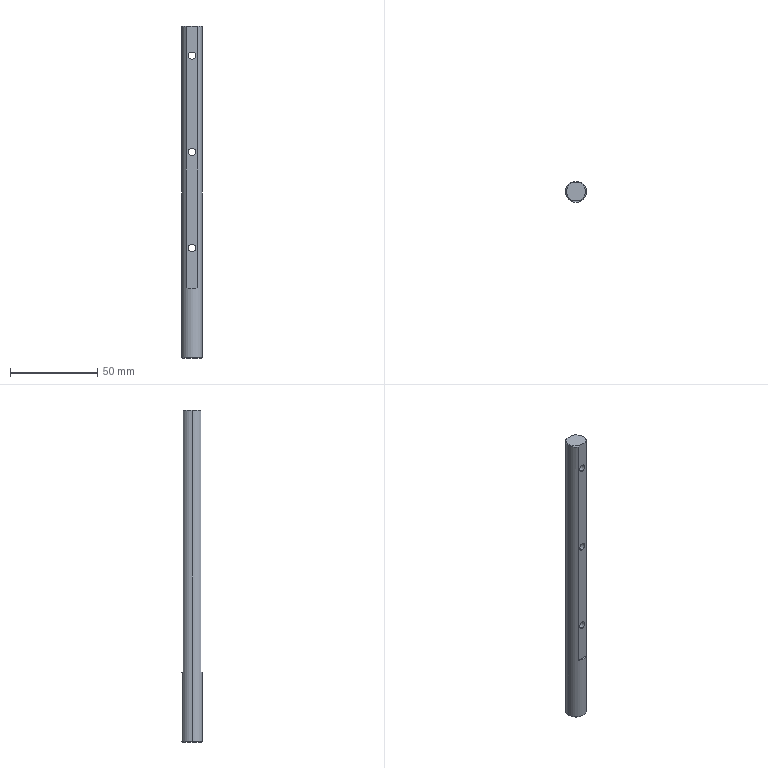Part | STEP file | 11-FG-S00411 | 1 solid | 19 faces | box 12 x 12 x 190 mm | volume 19715 mm3 | cylinder 8 | plane 6 | cone 5 | commonest cylinder face diameters 4.2 x6 12 x2
STEP:
#1=CARTESIAN_POINT('',(0.,-5.,75.9));
#2=VERTEX_POINT('',#1);
#3=CARTESIAN_POINT('',(0.,-5.,80.1));
#4=VERTEX_POINT('',#3);
#5=CARTESIAN_POINT('',(0.,-5.,78.));
#6=DIRECTION('',(0.,1.,0.));
#7=DIRECTION('',(0.,0.,1.));
#8=AXIS2_PLACEMENT_3D('',#5,#6,#7);
#9=CIRCLE('',#8,2.1);
#10=EDGE_CURVE('',#2,#4,#9,.T.);
#11=ORIENTED_EDGE('',*,*,#10,.F.);
#12=CARTESIAN_POINT('',(0.,5.,75.9));
#13=VERTEX_POINT('',#12);
#14=CARTESIAN_POINT('',(0.,-123.,75.9));
#15=DIRECTION('',(0.,1.,0.));
#16=VECTOR('',#15,1000.);
#17=LINE('',#14,#16);
#18=EDGE_CURVE('',#2,#13,#17,.T.);
#19=ORIENTED_EDGE('',*,*,#18,.T.);
#20=CARTESIAN_POINT('',(0.,5.,80.1));
#21=VERTEX_POINT('',#20);
#22=CARTESIAN_POINT('',(0.,5.,78.));
#23=DIRECTION('',(0.,1.,0.));
#24=DIRECTION('',(0.,0.,1.));
#25=AXIS2_PLACEMENT_3D('',#22,#23,#24);
#26=CIRCLE('',#25,2.1);
#27=EDGE_CURVE('',#13,#21,#26,.T.);
#28=ORIENTED_EDGE('',*,*,#27,.T.);
#29=CARTESIAN_POINT('',(0.,-123.,80.1));
#30=DIRECTION('',(0.,1.,0.));
#31=VECTOR('',#30,1000.);
#32=LINE('',#29,#31);
#33=EDGE_CURVE('',#4,#21,#32,.T.);
#34=ORIENTED_EDGE('',*,*,#33,.F.);
#35=EDGE_LOOP('',(#11,#19,#28,#34));
#36=FACE_OUTER_BOUND('',#35,.T.);
#37=CARTESIAN_POINT('',(0.,-123.,78.));
#38=DIRECTION('',(0.,1.,0.));
#39=DIRECTION('',(0.,0.,1.));
#40=AXIS2_PLACEMENT_3D('',#37,#38,#39);
#41=CYLINDRICAL_SURFACE('',#40,2.1);
#42=ADVANCED_FACE('',(#36),#41,.F.);
#43=CARTESIAN_POINT('',(0.,-5.,20.9));
#44=VERTEX_POINT('',#43);
#45=CARTESIAN_POINT('',(0.,-5.,25.1));
#46=VERTEX_POINT('',#45);
#47=CARTESIAN_POINT('',(0.,-5.,23.));
#48=DIRECTION('',(0.,1.,0.));
#49=DIRECTION('',(0.,0.,1.));
#50=AXIS2_PLACEMENT_3D('',#47,#48,#49);
#51=CIRCLE('',#50,2.1);
#52=EDGE_CURVE('',#44,#46,#51,.T.);
#53=ORIENTED_EDGE('',*,*,#52,.F.);
#54=CARTESIAN_POINT('',(0.,5.,20.9));
#55=VERTEX_POINT('',#54);
#56=CARTESIAN_POINT('',(0.,-123.,20.9));
#57=DIRECTION('',(0.,1.,0.));
#58=VECTOR('',#57,1000.);
#59=LINE('',#56,#58);
#60=EDGE_CURVE('',#44,#55,#59,.T.);
#61=ORIENTED_EDGE('',*,*,#60,.T.);
#62=CARTESIAN_POINT('',(0.,5.,25.1));
#63=VERTEX_POINT('',#62);
#64=CARTESIAN_POINT('',(0.,5.,23.));
#65=DIRECTION('',(0.,1.,0.));
#66=DIRECTION('',(0.,0.,1.));
#67=AXIS2_PLACEMENT_3D('',#64,#65,#66);
#68=CIRCLE('',#67,2.1);
#69=EDGE_CURVE('',#55,#63,#68,.T.);
#70=ORIENTED_EDGE('',*,*,#69,.T.);
#71=CARTESIAN_POINT('',(0.,-123.,25.1));
#72=DIRECTION('',(0.,1.,0.));
#73=VECTOR('',#72,1000.);
#74=LINE('',#71,#73);
#75=EDGE_CURVE('',#46,#63,#74,.T.);
#76=ORIENTED_EDGE('',*,*,#75,.F.);
#77=EDGE_LOOP('',(#53,#61,#70,#76));
#78=FACE_OUTER_BOUND('',#77,.T.);
#79=CARTESIAN_POINT('',(0.,-123.,23.));
#80=DIRECTION('',(0.,1.,0.));
#81=DIRECTION('',(0.,0.,1.));
#82=AXIS2_PLACEMENT_3D('',#79,#80,#81);
#83=CYLINDRICAL_SURFACE('',#82,2.1);
#84=ADVANCED_FACE('',(#78),#83,.F.);
#85=CARTESIAN_POINT('',(0.,-5.,-34.1));
#86=VERTEX_POINT('',#85);
#87=CARTESIAN_POINT('',(0.,-5.,-29.9));
#88=VERTEX_POINT('',#87);
#89=CARTESIAN_POINT('',(0.,-5.,-32.));
#90=DIRECTION('',(0.,1.,0.));
#91=DIRECTION('',(0.,0.,1.));
#92=AXIS2_PLACEMENT_3D('',#89,#90,#91);
#93=CIRCLE('',#92,2.1);
#94=EDGE_CURVE('',#86,#88,#93,.T.);
#95=ORIENTED_EDGE('',*,*,#94,.F.);
#96=CARTESIAN_POINT('',(0.,5.,-34.1));
#97=VERTEX_POINT('',#96);
#98=CARTESIAN_POINT('',(0.,-123.,-34.1));
#99=DIRECTION('',(0.,1.,0.));
#100=VECTOR('',#99,1000.);
#101=LINE('',#98,#100);
#102=EDGE_CURVE('',#86,#97,#101,.T.);
#103=ORIENTED_EDGE('',*,*,#102,.T.);
#104=CARTESIAN_POINT('',(0.,5.,-29.9));
#105=VERTEX_POINT('',#104);
#106=CARTESIAN_POINT('',(0.,5.,-32.));
#107=DIRECTION('',(0.,1.,0.));
#108=DIRECTION('',(0.,0.,1.));
#109=AXIS2_PLACEMENT_3D('',#106,#107,#108);
#110=CIRCLE('',#109,2.1);
#111=EDGE_CURVE('',#97,#105,#110,.T.);
#112=ORIENTED_EDGE('',*,*,#111,.T.);
#113=CARTESIAN_POINT('',(0.,-123.,-29.9));
#114=DIRECTION('',(0.,1.,0.));
#115=VECTOR('',#114,1000.);
#116=LINE('',#113,#115);
#117=EDGE_CURVE('',#88,#105,#116,.T.);
#118=ORIENTED_EDGE('',*,*,#117,.F.);
#119=EDGE_LOOP('',(#95,#103,#112,#118));
#120=FACE_OUTER_BOUND('',#119,.T.);
#121=CARTESIAN_POINT('',(0.,-123.,-32.));
#122=DIRECTION('',(0.,1.,0.));
#123=DIRECTION('',(0.,0.,1.));
#124=AXIS2_PLACEMENT_3D('',#121,#122,#123);
#125=CYLINDRICAL_SURFACE('',#124,2.1);
#126=ADVANCED_FACE('',(#120),#125,.F.);
#127=CARTESIAN_POINT('',(-5.5,0.,-95.));
#128=VERTEX_POINT('',#127);
#129=CARTESIAN_POINT('',(5.5,0.,-95.));
#130=VERTEX_POINT('',#129);
#131=CARTESIAN_POINT('',(0.,0.,-95.));
#132=DIRECTION('',(0.,0.,-1.));
#133=DIRECTION('',(1.,0.,0.));
#134=AXIS2_PLACEMENT_3D('',#131,#132,#133);
#135=CIRCLE('',#134,5.5);
#136=EDGE_CURVE('',#128,#130,#135,.T.);
#137=ORIENTED_EDGE('',*,*,#136,.F.);
#138=CARTESIAN_POINT('',(-6.,0.,-94.5));
#139=VERTEX_POINT('',#138);
#140=CARTESIAN_POINT('',(-6.,0.,-94.5));
#141=DIRECTION('',(-0.7071,0.,0.7071));
#142=VECTOR('',#141,1000.);
#143=LINE('',#140,#142);
#144=EDGE_CURVE('',#128,#139,#143,.T.);
#145=ORIENTED_EDGE('',*,*,#144,.T.);
#146=CARTESIAN_POINT('',(6.,0.,-94.5));
#147=VERTEX_POINT('',#146);
#148=CARTESIAN_POINT('',(0.,0.,-94.5));
#149=DIRECTION('',(0.,0.,1.));
#150=DIRECTION('',(1.,0.,0.));
#151=AXIS2_PLACEMENT_3D('',#148,#149,#150);
#152=CIRCLE('',#151,6.);
#153=EDGE_CURVE('',#147,#139,#152,.T.);
#154=ORIENTED_EDGE('',*,*,#153,.F.);
#155=CARTESIAN_POINT('',(6.,0.,-94.5));
#156=DIRECTION('',(0.7071,0.,0.7071));
#157=VECTOR('',#156,1000.);
#158=LINE('',#155,#157);
#159=EDGE_CURVE('',#130,#147,#158,.T.);
#160=ORIENTED_EDGE('',*,*,#159,.F.);
#161=EDGE_LOOP('',(#137,#145,#154,#160));
#162=FACE_OUTER_BOUND('',#161,.T.);
#163=CARTESIAN_POINT('',(0.,0.,-94.5));
#164=DIRECTION('',(0.,0.,1.));
#165=DIRECTION('',(1.,0.,0.));
#166=AXIS2_PLACEMENT_3D('',#163,#164,#165);
#167=CONICAL_SURFACE('',#166,6.,0.7854);
#168=ADVANCED_FACE('',(#162),#167,.T.);
#169=CARTESIAN_POINT('',(-5.5,0.,95.));
#170=VERTEX_POINT('',#169);
#171=CARTESIAN_POINT('',(-2.291,-5.,95.));
#172=VERTEX_POINT('',#171);
#173=CARTESIAN_POINT('',(0.,0.,95.));
#174=DIRECTION('',(0.,0.,1.));
#175=DIRECTION('',(1.,0.,0.));
#176=AXIS2_PLACEMENT_3D('',#173,#174,#175);
#177=CIRCLE('',#176,5.5);
#178=EDGE_CURVE('',#170,#172,#177,.T.);
#179=ORIENTED_EDGE('',*,*,#178,.F.);
#180=CARTESIAN_POINT('',(-6.,0.,94.5));
#181=VERTEX_POINT('',#180);
#182=CARTESIAN_POINT('',(-5.5,0.,95.));
#183=DIRECTION('',(-0.7071,0.,-0.7071));
#184=VECTOR('',#183,1000.);
#185=LINE('',#182,#184);
#186=EDGE_CURVE('',#170,#181,#185,.T.);
#187=ORIENTED_EDGE('',*,*,#186,.T.);
#188=CARTESIAN_POINT('',(-3.317,-5.,94.5));
#189=VERTEX_POINT('',#188);
#190=CARTESIAN_POINT('',(0.,0.,94.5));
#191=DIRECTION('',(0.,0.,-1.));
#192=DIRECTION('',(1.,0.,0.));
#193=AXIS2_PLACEMENT_3D('',#190,#191,#192);
#194=CIRCLE('',#193,6.);
#195=EDGE_CURVE('',#189,#181,#194,.T.);
#196=ORIENTED_EDGE('',*,*,#195,.F.);
#197=CARTESIAN_POINT('',(-2.291,-5.,95.));
#198=CARTESIAN_POINT('',(-2.645,-5.,94.853));
#199=CARTESIAN_POINT('',(-2.985,-5.,94.683));
#200=CARTESIAN_POINT('',(-3.317,-5.,94.5));
#201=B_SPLINE_CURVE_WITH_KNOTS('',3,(#197,#198,#199,#200),.UNSPECIFIED.,.F.,.F.,(4,4),(0.01077,0.01192),.UNSPECIFIED.);
#202=EDGE_CURVE('',#172,#189,#201,.T.);
#203=ORIENTED_EDGE('',*,*,#202,.F.);
#204=EDGE_LOOP('',(#179,#187,#196,#203));
#205=FACE_OUTER_BOUND('',#204,.T.);
#206=CARTESIAN_POINT('',(0.,0.,95.));
#207=DIRECTION('',(0.,0.,-1.));
#208=DIRECTION('',(-1.,0.,0.));
#209=AXIS2_PLACEMENT_3D('',#206,#207,#208);
#210=CONICAL_SURFACE('',#209,5.5,0.7854);
#211=ADVANCED_FACE('',(#205),#210,.T.);
#212=CARTESIAN_POINT('',(3.317,5.,94.5));
#213=VERTEX_POINT('',#212);
#214=CARTESIAN_POINT('',(6.,0.,94.5));
#215=VERTEX_POINT('',#214);
#216=CARTESIAN_POINT('',(0.,0.,94.5));
#217=DIRECTION('',(0.,0.,-1.));
#218=DIRECTION('',(1.,0.,0.));
#219=AXIS2_PLACEMENT_3D('',#216,#217,#218);
#220=CIRCLE('',#219,6.);
#221=EDGE_CURVE('',#213,#215,#220,.T.);
#222=ORIENTED_EDGE('',*,*,#221,.T.);
#223=CARTESIAN_POINT('',(6.,0.,95.));
#224=DIRECTION('',(0.,0.,-1.));
#225=VECTOR('',#224,1000.);
#226=LINE('',#223,#225);
#227=EDGE_CURVE('',#215,#147,#226,.T.);
#228=ORIENTED_EDGE('',*,*,#227,.T.);
#229=ORIENTED_EDGE('',*,*,#153,.T.);
#230=CARTESIAN_POINT('',(-6.,0.,95.));
#231=DIRECTION('',(0.,0.,-1.));
#232=VECTOR('',#231,1000.);
#233=LINE('',#230,#232);
#234=EDGE_CURVE('',#181,#139,#233,.T.);
#235=ORIENTED_EDGE('',*,*,#234,.F.);
#236=CARTESIAN_POINT('',(-3.317,5.,94.5));
#237=VERTEX_POINT('',#236);
#238=CARTESIAN_POINT('',(0.,0.,94.5));
#239=DIRECTION('',(0.,0.,-1.));
#240=DIRECTION('',(1.,0.,0.));
#241=AXIS2_PLACEMENT_3D('',#238,#239,#240);
#242=CIRCLE('',#241,6.);
#243=EDGE_CURVE('',#181,#237,#242,.T.);
#244=ORIENTED_EDGE('',*,*,#243,.T.);
#245=CARTESIAN_POINT('',(-3.317,5.,-55.));
#246=VERTEX_POINT('',#245);
#247=CARTESIAN_POINT('',(-3.317,5.,-55.));
#248=DIRECTION('',(0.,0.,1.));
#249=VECTOR('',#248,1000.);
#250=LINE('',#247,#249);
#251=EDGE_CURVE('',#246,#237,#250,.T.);
#252=ORIENTED_EDGE('',*,*,#251,.F.);
#253=CARTESIAN_POINT('',(3.317,5.,-55.));
#254=VERTEX_POINT('',#253);
#255=CARTESIAN_POINT('',(0.,0.,-55.));
#256=DIRECTION('',(0.,0.,1.));
#257=DIRECTION('',(1.,0.,0.));
#258=AXIS2_PLACEMENT_3D('',#255,#256,#257);
#259=CIRCLE('',#258,6.);
#260=EDGE_CURVE('',#254,#246,#259,.T.);
#261=ORIENTED_EDGE('',*,*,#260,.F.);
#262=CARTESIAN_POINT('',(3.317,5.,-55.));
#263=DIRECTION('',(0.,0.,1.));
#264=VECTOR('',#263,1000.);
#265=LINE('',#262,#264);
#266=EDGE_CURVE('',#254,#213,#265,.T.);
#267=ORIENTED_EDGE('',*,*,#266,.T.);
#268=EDGE_LOOP('',(#222,#228,#229,#235,#244,#252,#261,#267));
#269=FACE_OUTER_BOUND('',#268,.T.);
#270=CARTESIAN_POINT('',(0.,0.,95.));
#271=DIRECTION('',(0.,0.,-1.));
#272=DIRECTION('',(-1.,0.,0.));
#273=AXIS2_PLACEMENT_3D('',#270,#271,#272);
#274=CYLINDRICAL_SURFACE('',#273,6.);
#275=ADVANCED_FACE('',(#269),#274,.T.);
#276=CARTESIAN_POINT('',(3.317,-5.,94.5));
#277=VERTEX_POINT('',#276);
#278=CARTESIAN_POINT('',(2.291,-5.,95.));
#279=VERTEX_POINT('',#278);
#280=CARTESIAN_POINT('',(3.317,-5.,94.5));
#281=CARTESIAN_POINT('',(2.983,-5.,94.684));
#282=CARTESIAN_POINT('',(2.643,-5.,94.854));
#283=CARTESIAN_POINT('',(2.291,-5.,95.));
#284=B_SPLINE_CURVE_WITH_KNOTS('',3,(#280,#281,#282,#283),.UNSPECIFIED.,.F.,.F.,(4,4),(0.004911,0.006055),.UNSPECIFIED.);
#285=EDGE_CURVE('',#277,#279,#284,.T.);
#286=ORIENTED_EDGE('',*,*,#285,.F.);
#287=CARTESIAN_POINT('',(0.,0.,94.5));
#288=DIRECTION('',(0.,0.,-1.));
#289=DIRECTION('',(1.,0.,0.));
#290=AXIS2_PLACEMENT_3D('',#287,#288,#289);
#291=CIRCLE('',#290,6.);
#292=EDGE_CURVE('',#215,#277,#291,.T.);
#293=ORIENTED_EDGE('',*,*,#292,.F.);
#294=ORIENTED_EDGE('',*,*,#221,.F.);
#295=CARTESIAN_POINT('',(2.291,5.,95.));
#296=VERTEX_POINT('',#295);
#297=CARTESIAN_POINT('',(2.291,5.,95.));
#298=CARTESIAN_POINT('',(2.645,5.,94.853));
#299=CARTESIAN_POINT('',(2.985,5.,94.683));
#300=CARTESIAN_POINT('',(3.317,5.,94.5));
#301=B_SPLINE_CURVE_WITH_KNOTS('',3,(#297,#298,#299,#300),.UNSPECIFIED.,.F.,.F.,(4,4),(0.01077,0.01192),.UNSPECIFIED.);
#302=EDGE_CURVE('',#296,#213,#301,.T.);
#303=ORIENTED_EDGE('',*,*,#302,.F.);
#304=CARTESIAN_POINT('',(0.,0.,95.));
#305=DIRECTION('',(0.,0.,1.));
#306=DIRECTION('',(1.,0.,0.));
#307=AXIS2_PLACEMENT_3D('',#304,#305,#306);
#308=CIRCLE('',#307,5.5);
#309=EDGE_CURVE('',#279,#296,#308,.T.);
#310=ORIENTED_EDGE('',*,*,#309,.F.);
#311=EDGE_LOOP('',(#286,#293,#294,#303,#310));
#312=FACE_OUTER_BOUND('',#311,.T.);
#313=CARTESIAN_POINT('',(0.,0.,95.));
#314=DIRECTION('',(0.,0.,-1.));
#315=DIRECTION('',(-1.,0.,0.));
#316=AXIS2_PLACEMENT_3D('',#313,#314,#315);
#317=CONICAL_SURFACE('',#316,5.5,0.7854);
#318=ADVANCED_FACE('',(#312),#317,.T.);
#319=ORIENTED_EDGE('',*,*,#227,.F.);
#320=ORIENTED_EDGE('',*,*,#292,.T.);
#321=CARTESIAN_POINT('',(3.317,-5.,-55.));
#322=VERTEX_POINT('',#321);
#323=CARTESIAN_POINT('',(3.317,-5.,-55.));
#324=DIRECTION('',(0.,0.,1.));
#325=VECTOR('',#324,1000.);
#326=LINE('',#323,#325);
#327=EDGE_CURVE('',#322,#277,#326,.T.);
#328=ORIENTED_EDGE('',*,*,#327,.F.);
#329=CARTESIAN_POINT('',(-3.317,-5.,-55.));
#330=VERTEX_POINT('',#329);
#331=CARTESIAN_POINT('',(0.,0.,-55.));
#332=DIRECTION('',(0.,0.,1.));
#333=DIRECTION('',(1.,0.,0.));
#334=AXIS2_PLACEMENT_3D('',#331,#332,#333);
#335=CIRCLE('',#334,6.);
#336=EDGE_CURVE('',#330,#322,#335,.T.);
#337=ORIENTED_EDGE('',*,*,#336,.F.);
#338=CARTESIAN_POINT('',(-3.317,-5.,-55.));
#339=DIRECTION('',(0.,0.,1.));
#340=VECTOR('',#339,1000.);
#341=LINE('',#338,#340);
#342=EDGE_CURVE('',#330,#189,#341,.T.);
#343=ORIENTED_EDGE('',*,*,#342,.T.);
#344=ORIENTED_EDGE('',*,*,#195,.T.);
#345=ORIENTED_EDGE('',*,*,#234,.T.);
#346=CARTESIAN_POINT('',(0.,0.,-94.5));
#347=DIRECTION('',(0.,0.,1.));
#348=DIRECTION('',(1.,0.,0.));
#349=AXIS2_PLACEMENT_3D('',#346,#347,#348);
#350=CIRCLE('',#349,6.);
#351=EDGE_CURVE('',#139,#147,#350,.T.);
#352=ORIENTED_EDGE('',*,*,#351,.T.);
#353=EDGE_LOOP('',(#319,#320,#328,#337,#343,#344,#345,#352));
#354=FACE_OUTER_BOUND('',#353,.T.);
#355=CARTESIAN_POINT('',(0.,0.,95.));
#356=DIRECTION('',(0.,0.,-1.));
#357=DIRECTION('',(-1.,0.,0.));
#358=AXIS2_PLACEMENT_3D('',#355,#356,#357);
#359=CYLINDRICAL_SURFACE('',#358,6.);
#360=ADVANCED_FACE('',(#354),#359,.T.);
#361=CARTESIAN_POINT('',(-3.317,-5.,95.));
#362=DIRECTION('',(-1.,0.,0.));
#363=VECTOR('',#362,1000.);
#364=LINE('',#361,#363);
#365=EDGE_CURVE('',#279,#172,#364,.T.);
#366=ORIENTED_EDGE('',*,*,#365,.F.);
#367=ORIENTED_EDGE('',*,*,#309,.T.);
#368=CARTESIAN_POINT('',(-2.291,5.,95.));
#369=VERTEX_POINT('',#368);
#370=CARTESIAN_POINT('',(-3.317,5.,95.));
#371=DIRECTION('',(1.,0.,0.));
#372=VECTOR('',#371,1000.);
#373=LINE('',#370,#372);
#374=EDGE_CURVE('',#369,#296,#373,.T.);
#375=ORIENTED_EDGE('',*,*,#374,.F.);
#376=CARTESIAN_POINT('',(0.,0.,95.));
#377=DIRECTION('',(0.,0.,1.));
#378=DIRECTION('',(1.,0.,0.));
#379=AXIS2_PLACEMENT_3D('',#376,#377,#378);
#380=CIRCLE('',#379,5.5);
#381=EDGE_CURVE('',#369,#170,#380,.T.);
#382=ORIENTED_EDGE('',*,*,#381,.T.);
#383=ORIENTED_EDGE('',*,*,#178,.T.);
#384=EDGE_LOOP('',(#366,#367,#375,#382,#383));
#385=FACE_OUTER_BOUND('',#384,.T.);
#386=CARTESIAN_POINT('',(0.,0.,95.));
#387=DIRECTION('',(0.,0.,1.));
#388=DIRECTION('',(1.,0.,0.));
#389=AXIS2_PLACEMENT_3D('',#386,#387,#388);
#390=PLANE('',#389);
#391=ADVANCED_FACE('',(#385),#390,.T.);
#392=CARTESIAN_POINT('',(0.,0.,-95.));
#393=DIRECTION('',(0.,0.,-1.));
#394=DIRECTION('',(1.,0.,0.));
#395=AXIS2_PLACEMENT_3D('',#392,#393,#394);
#396=CIRCLE('',#395,5.5);
#397=EDGE_CURVE('',#130,#128,#396,.T.);
#398=ORIENTED_EDGE('',*,*,#397,.T.);
#399=ORIENTED_EDGE('',*,*,#136,.T.);
#400=EDGE_LOOP('',(#398,#399));
#401=FACE_OUTER_BOUND('',#400,.T.);
#402=CARTESIAN_POINT('',(0.,0.,-95.));
#403=DIRECTION('',(0.,0.,1.));
#404=DIRECTION('',(1.,0.,0.));
#405=AXIS2_PLACEMENT_3D('',#402,#403,#404);
#406=PLANE('',#405);
#407=ADVANCED_FACE('',(#401),#406,.F.);
#408=ORIENTED_EDGE('',*,*,#186,.F.);
#409=ORIENTED_EDGE('',*,*,#381,.F.);
#410=CARTESIAN_POINT('',(-3.317,5.,94.5));
#411=CARTESIAN_POINT('',(-2.983,5.,94.684));
#412=CARTESIAN_POINT('',(-2.643,5.,94.854));
#413=CARTESIAN_POINT('',(-2.291,5.,95.));
#414=B_SPLINE_CURVE_WITH_KNOTS('',3,(#410,#411,#412,#413),.UNSPECIFIED.,.F.,.F.,(4,4),(0.004911,0.006055),.UNSPECIFIED.);
#415=EDGE_CURVE('',#237,#369,#414,.T.);
#416=ORIENTED_EDGE('',*,*,#415,.F.);
#417=ORIENTED_EDGE('',*,*,#243,.F.);
#418=EDGE_LOOP('',(#408,#409,#416,#417));
#419=FACE_OUTER_BOUND('',#418,.T.);
#420=CARTESIAN_POINT('',(0.,0.,95.));
#421=DIRECTION('',(0.,0.,-1.));
#422=DIRECTION('',(-1.,0.,0.));
#423=AXIS2_PLACEMENT_3D('',#420,#421,#422);
#424=CONICAL_SURFACE('',#423,5.5,0.7854);
#425=ADVANCED_FACE('',(#419),#424,.T.);
#426=ORIENTED_EDGE('',*,*,#144,.F.);
#427=ORIENTED_EDGE('',*,*,#397,.F.);
#428=ORIENTED_EDGE('',*,*,#159,.T.);
#429=ORIENTED_EDGE('',*,*,#351,.F.);
#430=EDGE_LOOP('',(#426,#427,#428,#429));
#431=FACE_OUTER_BOUND('',#430,.T.);
#432=CARTESIAN_POINT('',(0.,0.,-94.5));
#433=DIRECTION('',(0.,0.,1.));
#434=DIRECTION('',(1.,0.,0.));
#435=AXIS2_PLACEMENT_3D('',#432,#433,#434);
#436=CONICAL_SURFACE('',#435,6.,0.7854);
#437=ADVANCED_FACE('',(#431),#436,.T.);
#438=CARTESIAN_POINT('',(0.,5.,78.));
#439=DIRECTION('',(0.,1.,0.));
#440=DIRECTION('',(0.,0.,1.));
#441=AXIS2_PLACEMENT_3D('',#438,#439,#440);
#442=CIRCLE('',#441,2.1);
#443=EDGE_CURVE('',#21,#13,#442,.T.);
#444=ORIENTED_EDGE('',*,*,#443,.F.);
#445=ORIENTED_EDGE('',*,*,#27,.F.);
#446=EDGE_LOOP('',(#444,#445));
#447=FACE_BOUND('',#446,.T.);
#448=CARTESIAN_POINT('',(0.,5.,23.));
#449=DIRECTION('',(0.,1.,0.));
#450=DIRECTION('',(0.,0.,1.));
#451=AXIS2_PLACEMENT_3D('',#448,#449,#450);
#452=CIRCLE('',#451,2.1);
#453=EDGE_CURVE('',#63,#55,#452,.T.);
#454=ORIENTED_EDGE('',*,*,#453,.F.);
#455=ORIENTED_EDGE('',*,*,#69,.F.);
#456=EDGE_LOOP('',(#454,#455));
#457=FACE_BOUND('',#456,.T.);
#458=CARTESIAN_POINT('',(0.,5.,-32.));
#459=DIRECTION('',(0.,1.,0.));
#460=DIRECTION('',(0.,0.,1.));
#461=AXIS2_PLACEMENT_3D('',#458,#459,#460);
#462=CIRCLE('',#461,2.1);
#463=EDGE_CURVE('',#105,#97,#462,.T.);
#464=ORIENTED_EDGE('',*,*,#463,.F.);
#465=ORIENTED_EDGE('',*,*,#111,.F.);
#466=EDGE_LOOP('',(#464,#465));
#467=FACE_BOUND('',#466,.T.);
#468=ORIENTED_EDGE('',*,*,#415,.T.);
#469=ORIENTED_EDGE('',*,*,#374,.T.);
#470=ORIENTED_EDGE('',*,*,#302,.T.);
#471=ORIENTED_EDGE('',*,*,#266,.F.);
#472=CARTESIAN_POINT('',(-3.317,5.,-55.));
#473=DIRECTION('',(1.,0.,0.));
#474=VECTOR('',#473,1000.);
#475=LINE('',#472,#474);
#476=EDGE_CURVE('',#246,#254,#475,.T.);
#477=ORIENTED_EDGE('',*,*,#476,.F.);
#478=ORIENTED_EDGE('',*,*,#251,.T.);
#479=EDGE_LOOP('',(#468,#469,#470,#471,#477,#478));
#480=FACE_OUTER_BOUND('',#479,.T.);
#481=CARTESIAN_POINT('',(-3.317,5.,-55.));
#482=DIRECTION('',(0.,-1.,0.));
#483=DIRECTION('',(0.,0.,-1.));
#484=AXIS2_PLACEMENT_3D('',#481,#482,#483);
#485=PLANE('',#484);
#486=ADVANCED_FACE('',(#447,#457,#467,#480),#485,.F.);
#487=ORIENTED_EDGE('',*,*,#260,.T.);
#488=ORIENTED_EDGE('',*,*,#476,.T.);
#489=EDGE_LOOP('',(#487,#488));
#490=FACE_OUTER_BOUND('',#489,.T.);
#491=CARTESIAN_POINT('',(0.,0.,-55.));
#492=DIRECTION('',(0.,0.,1.));
#493=DIRECTION('',(1.,0.,0.));
#494=AXIS2_PLACEMENT_3D('',#491,#492,#493);
#495=PLANE('',#494);
#496=ADVANCED_FACE('',(#490),#495,.T.);
#497=CARTESIAN_POINT('',(0.,-5.,78.));
#498=DIRECTION('',(0.,1.,0.));
#499=DIRECTION('',(0.,0.,1.));
#500=AXIS2_PLACEMENT_3D('',#497,#498,#499);
#501=CIRCLE('',#500,2.1);
#502=EDGE_CURVE('',#4,#2,#501,.T.);
#503=ORIENTED_EDGE('',*,*,#502,.T.);
#504=ORIENTED_EDGE('',*,*,#10,.T.);
#505=EDGE_LOOP('',(#503,#504));
#506=FACE_BOUND('',#505,.T.);
#507=CARTESIAN_POINT('',(0.,-5.,23.));
#508=DIRECTION('',(0.,1.,0.));
#509=DIRECTION('',(0.,0.,1.));
#510=AXIS2_PLACEMENT_3D('',#507,#508,#509);
#511=CIRCLE('',#510,2.1);
#512=EDGE_CURVE('',#46,#44,#511,.T.);
#513=ORIENTED_EDGE('',*,*,#512,.T.);
#514=ORIENTED_EDGE('',*,*,#52,.T.);
#515=EDGE_LOOP('',(#513,#514));
#516=FACE_BOUND('',#515,.T.);
#517=CARTESIAN_POINT('',(0.,-5.,-32.));
#518=DIRECTION('',(0.,1.,0.));
#519=DIRECTION('',(0.,0.,1.));
#520=AXIS2_PLACEMENT_3D('',#517,#518,#519);
#521=CIRCLE('',#520,2.1);
#522=EDGE_CURVE('',#88,#86,#521,.T.);
#523=ORIENTED_EDGE('',*,*,#522,.T.);
#524=ORIENTED_EDGE('',*,*,#94,.T.);
#525=EDGE_LOOP('',(#523,#524));
#526=FACE_BOUND('',#525,.T.);
#527=ORIENTED_EDGE('',*,*,#285,.T.);
#528=ORIENTED_EDGE('',*,*,#365,.T.);
#529=ORIENTED_EDGE('',*,*,#202,.T.);
#530=ORIENTED_EDGE('',*,*,#342,.F.);
#531=CARTESIAN_POINT('',(-3.317,-5.,-55.));
#532=DIRECTION('',(-1.,0.,0.));
#533=VECTOR('',#532,1000.);
#534=LINE('',#531,#533);
#535=EDGE_CURVE('',#322,#330,#534,.T.);
#536=ORIENTED_EDGE('',*,*,#535,.F.);
#537=ORIENTED_EDGE('',*,*,#327,.T.);
#538=EDGE_LOOP('',(#527,#528,#529,#530,#536,#537));
#539=FACE_OUTER_BOUND('',#538,.T.);
#540=CARTESIAN_POINT('',(-3.317,-5.,-55.));
#541=DIRECTION('',(0.,1.,0.));
#542=DIRECTION('',(0.,0.,1.));
#543=AXIS2_PLACEMENT_3D('',#540,#541,#542);
#544=PLANE('',#543);
#545=ADVANCED_FACE('',(#506,#516,#526,#539),#544,.F.);
#546=ORIENTED_EDGE('',*,*,#336,.T.);
#547=ORIENTED_EDGE('',*,*,#535,.T.);
#548=EDGE_LOOP('',(#546,#547));
#549=FACE_OUTER_BOUND('',#548,.T.);
#550=CARTESIAN_POINT('',(0.,0.,-55.));
#551=DIRECTION('',(0.,0.,1.));
#552=DIRECTION('',(1.,0.,0.));
#553=AXIS2_PLACEMENT_3D('',#550,#551,#552);
#554=PLANE('',#553);
#555=ADVANCED_FACE('',(#549),#554,.T.);
#556=ORIENTED_EDGE('',*,*,#102,.F.);
#557=ORIENTED_EDGE('',*,*,#522,.F.);
#558=ORIENTED_EDGE('',*,*,#117,.T.);
#559=ORIENTED_EDGE('',*,*,#463,.T.);
#560=EDGE_LOOP('',(#556,#557,#558,#559));
#561=FACE_OUTER_BOUND('',#560,.T.);
#562=CARTESIAN_POINT('',(0.,-123.,-32.));
#563=DIRECTION('',(0.,1.,0.));
#564=DIRECTION('',(0.,0.,1.));
#565=AXIS2_PLACEMENT_3D('',#562,#563,#564);
#566=CYLINDRICAL_SURFACE('',#565,2.1);
#567=ADVANCED_FACE('',(#561),#566,.F.);
#568=ORIENTED_EDGE('',*,*,#60,.F.);
#569=ORIENTED_EDGE('',*,*,#512,.F.);
#570=ORIENTED_EDGE('',*,*,#75,.T.);
#571=ORIENTED_EDGE('',*,*,#453,.T.);
#572=EDGE_LOOP('',(#568,#569,#570,#571));
#573=FACE_OUTER_BOUND('',#572,.T.);
#574=CARTESIAN_POINT('',(0.,-123.,23.));
#575=DIRECTION('',(0.,1.,0.));
#576=DIRECTION('',(0.,0.,1.));
#577=AXIS2_PLACEMENT_3D('',#574,#575,#576);
#578=CYLINDRICAL_SURFACE('',#577,2.1);
#579=ADVANCED_FACE('',(#573),#578,.F.);
#580=ORIENTED_EDGE('',*,*,#18,.F.);
#581=ORIENTED_EDGE('',*,*,#502,.F.);
#582=ORIENTED_EDGE('',*,*,#33,.T.);
#583=ORIENTED_EDGE('',*,*,#443,.T.);
#584=EDGE_LOOP('',(#580,#581,#582,#583));
#585=FACE_OUTER_BOUND('',#584,.T.);
#586=CARTESIAN_POINT('',(0.,-123.,78.));
#587=DIRECTION('',(0.,1.,0.));
#588=DIRECTION('',(0.,0.,1.));
#589=AXIS2_PLACEMENT_3D('',#586,#587,#588);
#590=CYLINDRICAL_SURFACE('',#589,2.1);
#591=ADVANCED_FACE('',(#585),#590,.F.);
#592=CLOSED_SHELL('',(#42,#84,#126,#168,#211,#275,#318,#360,#391,#407,#425,#437,#486,#496,#545,#555,#567,#579,#591));
#593=MANIFOLD_SOLID_BREP('',#592);
#594=CARTESIAN_POINT('',(0.,0.,0.));
#595=DIRECTION('',(0.,0.,1.));
#596=DIRECTION('',(1.,0.,0.));
#597=AXIS2_PLACEMENT_3D('',#594,#595,#596);
#598=(LENGTH_UNIT()NAMED_UNIT(*)SI_UNIT(.MILLI.,.METRE.));
#599=UNCERTAINTY_MEASURE_WITH_UNIT(LENGTH_MEASURE(0.00001),#598,'','');
#600=(NAMED_UNIT(*)PLANE_ANGLE_UNIT()SI_UNIT($,.RADIAN.));
#601=(NAMED_UNIT(*)SI_UNIT($,.STERADIAN.)SOLID_ANGLE_UNIT());
#602=(GEOMETRIC_REPRESENTATION_CONTEXT(3)GLOBAL_UNCERTAINTY_ASSIGNED_CONTEXT((#599))GLOBAL_UNIT_ASSIGNED_CONTEXT((#598,#600,#601))REPRESENTATION_CONTEXT('',''));
#603=ADVANCED_BREP_SHAPE_REPRESENTATION('',(#593,#597),#602);